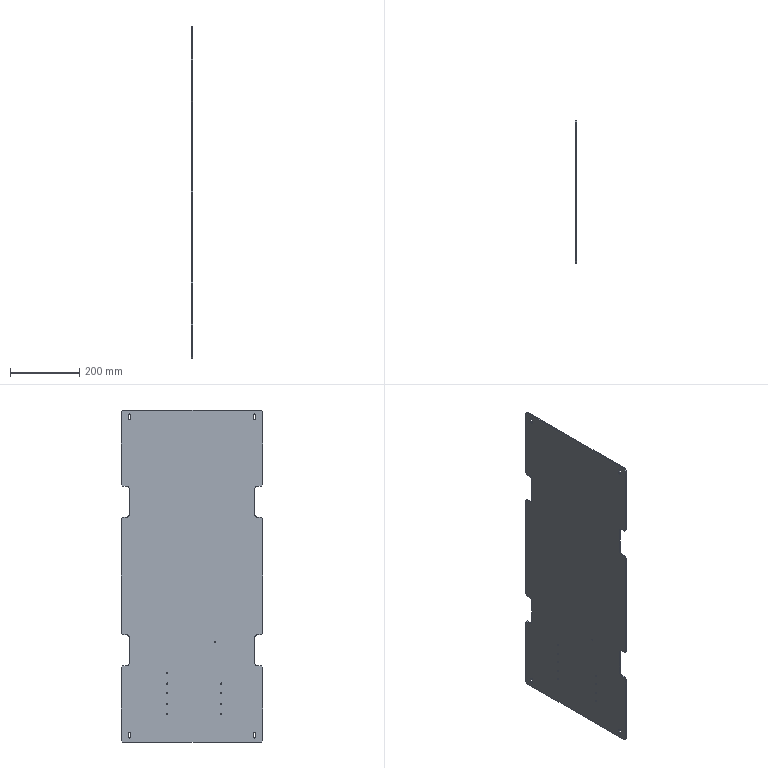Part | SolidWorks | features BaseBody 1 | 1 solid | 82 faces | box 3 x 410 x 960 mm | volume 1152307 mm3 | plane 42 | cylinder 40 | commonest cylinder face diameters 3.3 x20 7 x12 20 x8